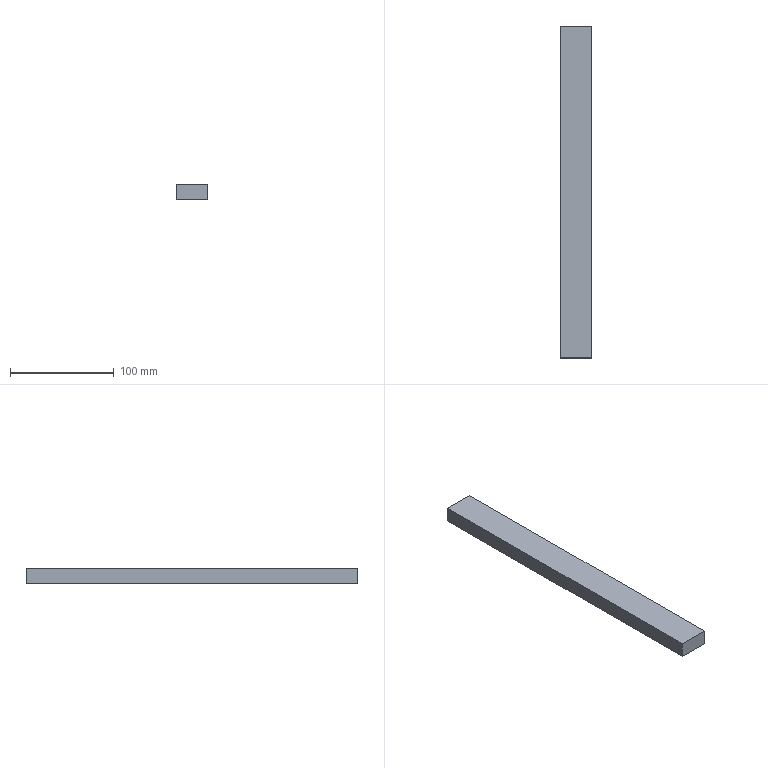Part | NX | features solid 2 | 1 solid | 6 faces | box 30 x 320 x 15 mm | volume 144000 mm3 | plane 6
STEP:
#1=CARTESIAN_POINT('',(-512.5,80.,-84.));
#2=VERTEX_POINT('',#1);
#3=CARTESIAN_POINT('',(-512.5,-240.,-84.));
#4=VERTEX_POINT('',#3);
#5=CARTESIAN_POINT('',(-512.5,40.,-84.));
#6=DIRECTION('',(0.,1.,0.));
#7=VECTOR('',#6,1000.);
#8=LINE('',#5,#7);
#9=EDGE_CURVE('',#2,#4,#8,.F.);
#10=ORIENTED_EDGE('',*,*,#9,.T.);
#11=CARTESIAN_POINT('',(-512.5,-240.,-69.));
#12=VERTEX_POINT('',#11);
#13=CARTESIAN_POINT('',(-512.5,-240.,-84.));
#14=DIRECTION('',(0.,0.,-1.));
#15=VECTOR('',#14,1000.);
#16=LINE('',#13,#15);
#17=EDGE_CURVE('',#4,#12,#16,.F.);
#18=ORIENTED_EDGE('',*,*,#17,.T.);
#19=CARTESIAN_POINT('',(-512.5,80.,-69.));
#20=VERTEX_POINT('',#19);
#21=CARTESIAN_POINT('',(-512.5,40.,-69.));
#22=DIRECTION('',(0.,1.,0.));
#23=VECTOR('',#22,1000.);
#24=LINE('',#21,#23);
#25=EDGE_CURVE('',#20,#12,#24,.F.);
#26=ORIENTED_EDGE('',*,*,#25,.F.);
#27=CARTESIAN_POINT('',(-512.5,80.,-84.));
#28=DIRECTION('',(0.,0.,-1.));
#29=VECTOR('',#28,1000.);
#30=LINE('',#27,#29);
#31=EDGE_CURVE('',#2,#20,#30,.F.);
#32=ORIENTED_EDGE('',*,*,#31,.F.);
#33=EDGE_LOOP('',(#10,#18,#26,#32));
#34=FACE_BOUND('',#33,.T.);
#35=CARTESIAN_POINT('',(-512.5,40.,-84.));
#36=DIRECTION('',(-1.,0.,0.));
#37=DIRECTION('',(0.,0.,1.));
#38=AXIS2_PLACEMENT_3D('',#35,#36,#37);
#39=PLANE('',#38);
#40=ADVANCED_FACE('',(#34),#39,.T.);
#41=ORIENTED_EDGE('',*,*,#25,.T.);
#42=CARTESIAN_POINT('',(-482.5,-240.,-69.));
#43=VERTEX_POINT('',#42);
#44=CARTESIAN_POINT('',(-512.5,-240.,-69.));
#45=DIRECTION('',(-1.,0.,0.));
#46=VECTOR('',#45,1000.);
#47=LINE('',#44,#46);
#48=EDGE_CURVE('',#12,#43,#47,.F.);
#49=ORIENTED_EDGE('',*,*,#48,.T.);
#50=CARTESIAN_POINT('',(-482.5,80.,-69.));
#51=VERTEX_POINT('',#50);
#52=CARTESIAN_POINT('',(-482.5,40.,-69.));
#53=DIRECTION('',(0.,1.,0.));
#54=VECTOR('',#53,1000.);
#55=LINE('',#52,#54);
#56=EDGE_CURVE('',#51,#43,#55,.F.);
#57=ORIENTED_EDGE('',*,*,#56,.F.);
#58=CARTESIAN_POINT('',(-512.5,80.,-69.));
#59=DIRECTION('',(-1.,0.,0.));
#60=VECTOR('',#59,1000.);
#61=LINE('',#58,#60);
#62=EDGE_CURVE('',#20,#51,#61,.F.);
#63=ORIENTED_EDGE('',*,*,#62,.F.);
#64=EDGE_LOOP('',(#41,#49,#57,#63));
#65=FACE_BOUND('',#64,.T.);
#66=CARTESIAN_POINT('',(-512.5,40.,-69.));
#67=DIRECTION('',(0.,0.,1.));
#68=DIRECTION('',(1.,0.,0.));
#69=AXIS2_PLACEMENT_3D('',#66,#67,#68);
#70=PLANE('',#69);
#71=ADVANCED_FACE('',(#65),#70,.T.);
#72=ORIENTED_EDGE('',*,*,#56,.T.);
#73=CARTESIAN_POINT('',(-482.5,-240.,-84.));
#74=VERTEX_POINT('',#73);
#75=CARTESIAN_POINT('',(-482.5,-240.,-84.));
#76=DIRECTION('',(0.,0.,1.));
#77=VECTOR('',#76,1000.);
#78=LINE('',#75,#77);
#79=EDGE_CURVE('',#74,#43,#78,.T.);
#80=ORIENTED_EDGE('',*,*,#79,.F.);
#81=CARTESIAN_POINT('',(-482.5,80.,-84.));
#82=VERTEX_POINT('',#81);
#83=CARTESIAN_POINT('',(-482.5,40.,-84.));
#84=DIRECTION('',(0.,1.,0.));
#85=VECTOR('',#84,1000.);
#86=LINE('',#83,#85);
#87=EDGE_CURVE('',#82,#74,#86,.F.);
#88=ORIENTED_EDGE('',*,*,#87,.F.);
#89=CARTESIAN_POINT('',(-482.5,80.,-69.));
#90=DIRECTION('',(0.,0.,1.));
#91=VECTOR('',#90,1000.);
#92=LINE('',#89,#91);
#93=EDGE_CURVE('',#82,#51,#92,.T.);
#94=ORIENTED_EDGE('',*,*,#93,.T.);
#95=EDGE_LOOP('',(#72,#80,#88,#94));
#96=FACE_BOUND('',#95,.T.);
#97=CARTESIAN_POINT('',(-482.5,40.,-84.));
#98=DIRECTION('',(-1.,0.,0.));
#99=DIRECTION('',(0.,0.,1.));
#100=AXIS2_PLACEMENT_3D('',#97,#98,#99);
#101=PLANE('',#100);
#102=ADVANCED_FACE('',(#96),#101,.F.);
#103=CARTESIAN_POINT('',(-442.5,80.,-84.));
#104=DIRECTION('',(1.,0.,0.));
#105=VECTOR('',#104,1000.);
#106=LINE('',#103,#105);
#107=EDGE_CURVE('',#2,#82,#106,.T.);
#108=ORIENTED_EDGE('',*,*,#107,.T.);
#109=ORIENTED_EDGE('',*,*,#87,.T.);
#110=CARTESIAN_POINT('',(-512.5,-240.,-84.));
#111=DIRECTION('',(1.,0.,0.));
#112=VECTOR('',#111,1000.);
#113=LINE('',#110,#112);
#114=EDGE_CURVE('',#4,#74,#113,.T.);
#115=ORIENTED_EDGE('',*,*,#114,.F.);
#116=ORIENTED_EDGE('',*,*,#9,.F.);
#117=EDGE_LOOP('',(#108,#109,#115,#116));
#118=FACE_BOUND('',#117,.T.);
#119=CARTESIAN_POINT('',(-512.5,40.,-84.));
#120=DIRECTION('',(0.,0.,1.));
#121=DIRECTION('',(1.,0.,0.));
#122=AXIS2_PLACEMENT_3D('',#119,#120,#121);
#123=PLANE('',#122);
#124=ADVANCED_FACE('',(#118),#123,.F.);
#125=ORIENTED_EDGE('',*,*,#79,.T.);
#126=ORIENTED_EDGE('',*,*,#48,.F.);
#127=ORIENTED_EDGE('',*,*,#17,.F.);
#128=ORIENTED_EDGE('',*,*,#114,.T.);
#129=EDGE_LOOP('',(#125,#126,#127,#128));
#130=FACE_BOUND('',#129,.T.);
#131=CARTESIAN_POINT('',(-512.5,-240.,-84.));
#132=DIRECTION('',(0.,1.,0.));
#133=DIRECTION('',(0.,0.,1.));
#134=AXIS2_PLACEMENT_3D('',#131,#132,#133);
#135=PLANE('',#134);
#136=ADVANCED_FACE('',(#130),#135,.F.);
#137=ORIENTED_EDGE('',*,*,#93,.F.);
#138=ORIENTED_EDGE('',*,*,#107,.F.);
#139=ORIENTED_EDGE('',*,*,#31,.T.);
#140=ORIENTED_EDGE('',*,*,#62,.T.);
#141=EDGE_LOOP('',(#137,#138,#139,#140));
#142=FACE_BOUND('',#141,.T.);
#143=CARTESIAN_POINT('',(-442.5,80.,-69.));
#144=DIRECTION('',(0.,1.,0.));
#145=DIRECTION('',(0.,0.,1.));
#146=AXIS2_PLACEMENT_3D('',#143,#144,#145);
#147=PLANE('',#146);
#148=ADVANCED_FACE('',(#142),#147,.T.);
#149=CLOSED_SHELL('',(#40,#71,#102,#124,#136,#148));
#150=MANIFOLD_SOLID_BREP('',#149);
#151=(LENGTH_UNIT()NAMED_UNIT(*)SI_UNIT(.MILLI.,.METRE.));
#152=UNCERTAINTY_MEASURE_WITH_UNIT(LENGTH_MEASURE(0.00001),#151,'','');
#153=(NAMED_UNIT(*)PLANE_ANGLE_UNIT()SI_UNIT($,.RADIAN.));
#154=(NAMED_UNIT(*)SI_UNIT($,.STERADIAN.)SOLID_ANGLE_UNIT());
#155=(GEOMETRIC_REPRESENTATION_CONTEXT(3)GLOBAL_UNCERTAINTY_ASSIGNED_CONTEXT((#152))GLOBAL_UNIT_ASSIGNED_CONTEXT((#151,#153,#154))REPRESENTATION_CONTEXT('',''));
#156=ADVANCED_BREP_SHAPE_REPRESENTATION('',(#150),#155);